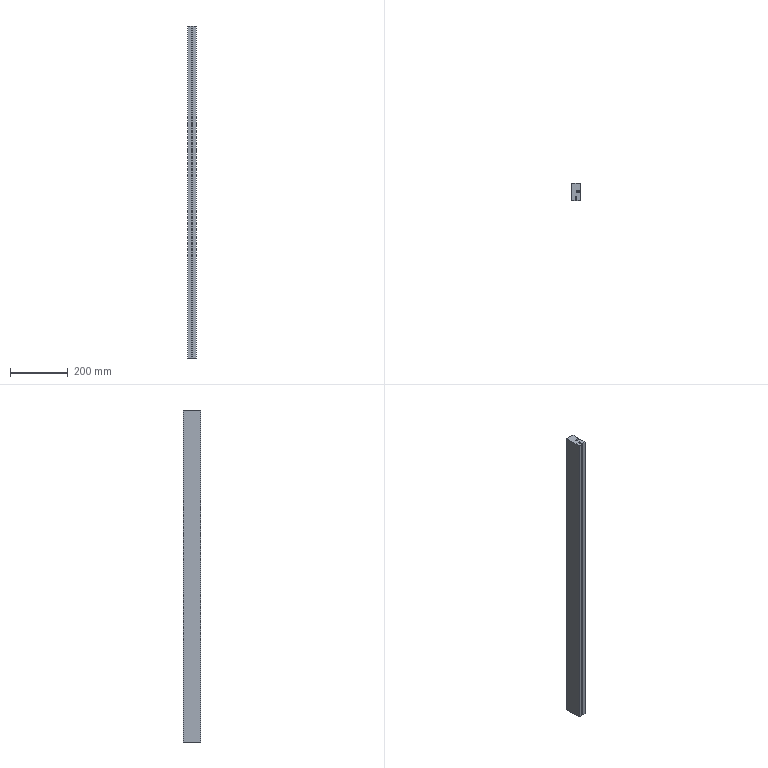Part | STEP file | 750038305 | 1 solid | 14 faces | box 30 x 60 x 1149 mm | volume 1861380 mm3 | plane 14
STEP:
#1=CARTESIAN_POINT('',(0.,0.,1149.));
#2=VERTEX_POINT('',#1);
#3=CARTESIAN_POINT('',(0.,0.,0.));
#4=VERTEX_POINT('',#3);
#5=CARTESIAN_POINT('',(0.,0.,1149.));
#6=DIRECTION('',(0.,0.,-1.));
#7=VECTOR('',#6,1000.);
#8=LINE('',#5,#7);
#9=EDGE_CURVE('',#2,#4,#8,.T.);
#10=ORIENTED_EDGE('',*,*,#9,.F.);
#11=CARTESIAN_POINT('',(0.,60.,1149.));
#12=VERTEX_POINT('',#11);
#13=CARTESIAN_POINT('',(0.,60.,1149.));
#14=DIRECTION('',(0.,-1.,0.));
#15=VECTOR('',#14,1000.);
#16=LINE('',#13,#15);
#17=EDGE_CURVE('',#12,#2,#16,.T.);
#18=ORIENTED_EDGE('',*,*,#17,.F.);
#19=CARTESIAN_POINT('',(0.,60.,0.));
#20=VERTEX_POINT('',#19);
#21=CARTESIAN_POINT('',(0.,60.,1149.));
#22=DIRECTION('',(0.,0.,1.));
#23=VECTOR('',#22,1000.);
#24=LINE('',#21,#23);
#25=EDGE_CURVE('',#20,#12,#24,.T.);
#26=ORIENTED_EDGE('',*,*,#25,.F.);
#27=CARTESIAN_POINT('',(0.,60.,0.));
#28=DIRECTION('',(0.,1.,0.));
#29=VECTOR('',#28,1000.);
#30=LINE('',#27,#29);
#31=EDGE_CURVE('',#4,#20,#30,.T.);
#32=ORIENTED_EDGE('',*,*,#31,.F.);
#33=EDGE_LOOP('',(#10,#18,#26,#32));
#34=FACE_OUTER_BOUND('',#33,.T.);
#35=CARTESIAN_POINT('',(0.,60.,1149.));
#36=DIRECTION('',(1.,0.,0.));
#37=DIRECTION('',(0.,0.,-1.));
#38=AXIS2_PLACEMENT_3D('',#35,#36,#37);
#39=PLANE('',#38);
#40=ADVANCED_FACE('',(#34),#39,.F.);
#41=CARTESIAN_POINT('',(15.,33.,0.));
#42=VERTEX_POINT('',#41);
#43=CARTESIAN_POINT('',(30.,33.,0.));
#44=VERTEX_POINT('',#43);
#45=CARTESIAN_POINT('',(0.,33.,0.));
#46=DIRECTION('',(1.,0.,0.));
#47=VECTOR('',#46,1000.);
#48=LINE('',#45,#47);
#49=EDGE_CURVE('',#42,#44,#48,.T.);
#50=ORIENTED_EDGE('',*,*,#49,.F.);
#51=CARTESIAN_POINT('',(15.,27.,0.));
#52=VERTEX_POINT('',#51);
#53=CARTESIAN_POINT('',(15.,0.,0.));
#54=DIRECTION('',(0.,1.,0.));
#55=VECTOR('',#54,1000.);
#56=LINE('',#53,#55);
#57=EDGE_CURVE('',#52,#42,#56,.T.);
#58=ORIENTED_EDGE('',*,*,#57,.F.);
#59=CARTESIAN_POINT('',(30.,27.,0.));
#60=VERTEX_POINT('',#59);
#61=CARTESIAN_POINT('',(0.,27.,0.));
#62=DIRECTION('',(-1.,0.,0.));
#63=VECTOR('',#62,1000.);
#64=LINE('',#61,#63);
#65=EDGE_CURVE('',#60,#52,#64,.T.);
#66=ORIENTED_EDGE('',*,*,#65,.F.);
#67=CARTESIAN_POINT('',(30.,0.,0.));
#68=VERTEX_POINT('',#67);
#69=CARTESIAN_POINT('',(30.,0.,0.));
#70=DIRECTION('',(0.,1.,0.));
#71=VECTOR('',#70,1000.);
#72=LINE('',#69,#71);
#73=EDGE_CURVE('',#68,#60,#72,.T.);
#74=ORIENTED_EDGE('',*,*,#73,.F.);
#75=CARTESIAN_POINT('',(18.,0.,0.));
#76=VERTEX_POINT('',#75);
#77=CARTESIAN_POINT('',(0.,0.,0.));
#78=DIRECTION('',(1.,0.,0.));
#79=VECTOR('',#78,1000.);
#80=LINE('',#77,#79);
#81=EDGE_CURVE('',#76,#68,#80,.T.);
#82=ORIENTED_EDGE('',*,*,#81,.F.);
#83=CARTESIAN_POINT('',(18.,15.,0.));
#84=VERTEX_POINT('',#83);
#85=CARTESIAN_POINT('',(18.,0.,0.));
#86=DIRECTION('',(0.,-1.,0.));
#87=VECTOR('',#86,1000.);
#88=LINE('',#85,#87);
#89=EDGE_CURVE('',#84,#76,#88,.T.);
#90=ORIENTED_EDGE('',*,*,#89,.F.);
#91=CARTESIAN_POINT('',(12.,15.,0.));
#92=VERTEX_POINT('',#91);
#93=CARTESIAN_POINT('',(0.,15.,0.));
#94=DIRECTION('',(1.,0.,0.));
#95=VECTOR('',#94,1000.);
#96=LINE('',#93,#95);
#97=EDGE_CURVE('',#92,#84,#96,.T.);
#98=ORIENTED_EDGE('',*,*,#97,.F.);
#99=CARTESIAN_POINT('',(12.,0.,0.));
#100=VERTEX_POINT('',#99);
#101=CARTESIAN_POINT('',(12.,0.,0.));
#102=DIRECTION('',(0.,1.,0.));
#103=VECTOR('',#102,1000.);
#104=LINE('',#101,#103);
#105=EDGE_CURVE('',#100,#92,#104,.T.);
#106=ORIENTED_EDGE('',*,*,#105,.F.);
#107=CARTESIAN_POINT('',(0.,0.,0.));
#108=DIRECTION('',(1.,0.,0.));
#109=VECTOR('',#108,1000.);
#110=LINE('',#107,#109);
#111=EDGE_CURVE('',#4,#100,#110,.T.);
#112=ORIENTED_EDGE('',*,*,#111,.F.);
#113=ORIENTED_EDGE('',*,*,#31,.T.);
#114=CARTESIAN_POINT('',(30.,60.,0.));
#115=VERTEX_POINT('',#114);
#116=CARTESIAN_POINT('',(0.,60.,0.));
#117=DIRECTION('',(-1.,0.,0.));
#118=VECTOR('',#117,1000.);
#119=LINE('',#116,#118);
#120=EDGE_CURVE('',#115,#20,#119,.T.);
#121=ORIENTED_EDGE('',*,*,#120,.F.);
#122=CARTESIAN_POINT('',(30.,0.,0.));
#123=DIRECTION('',(0.,1.,0.));
#124=VECTOR('',#123,1000.);
#125=LINE('',#122,#124);
#126=EDGE_CURVE('',#44,#115,#125,.T.);
#127=ORIENTED_EDGE('',*,*,#126,.F.);
#128=EDGE_LOOP('',(#50,#58,#66,#74,#82,#90,#98,#106,#112,#113,#121,#127));
#129=FACE_OUTER_BOUND('',#128,.T.);
#130=CARTESIAN_POINT('',(0.,0.,0.));
#131=DIRECTION('',(0.,0.,1.));
#132=DIRECTION('',(1.,0.,0.));
#133=AXIS2_PLACEMENT_3D('',#130,#131,#132);
#134=PLANE('',#133);
#135=ADVANCED_FACE('',(#129),#134,.F.);
#136=CARTESIAN_POINT('',(12.,0.,1149.));
#137=VERTEX_POINT('',#136);
#138=CARTESIAN_POINT('',(12.,0.,1149.));
#139=DIRECTION('',(0.,0.,-1.));
#140=VECTOR('',#139,1000.);
#141=LINE('',#138,#140);
#142=EDGE_CURVE('',#137,#100,#141,.T.);
#143=ORIENTED_EDGE('',*,*,#142,.F.);
#144=CARTESIAN_POINT('',(0.,0.,1149.));
#145=DIRECTION('',(1.,0.,0.));
#146=VECTOR('',#145,1000.);
#147=LINE('',#144,#146);
#148=EDGE_CURVE('',#2,#137,#147,.T.);
#149=ORIENTED_EDGE('',*,*,#148,.F.);
#150=ORIENTED_EDGE('',*,*,#9,.T.);
#151=ORIENTED_EDGE('',*,*,#111,.T.);
#152=EDGE_LOOP('',(#143,#149,#150,#151));
#153=FACE_OUTER_BOUND('',#152,.T.);
#154=CARTESIAN_POINT('',(0.,0.,1149.));
#155=DIRECTION('',(0.,1.,0.));
#156=DIRECTION('',(0.,0.,1.));
#157=AXIS2_PLACEMENT_3D('',#154,#155,#156);
#158=PLANE('',#157);
#159=ADVANCED_FACE('',(#153),#158,.F.);
#160=CARTESIAN_POINT('',(15.,27.,1149.));
#161=VERTEX_POINT('',#160);
#162=CARTESIAN_POINT('',(15.,33.,1149.));
#163=VERTEX_POINT('',#162);
#164=CARTESIAN_POINT('',(15.,0.,1149.));
#165=DIRECTION('',(0.,1.,0.));
#166=VECTOR('',#165,1000.);
#167=LINE('',#164,#166);
#168=EDGE_CURVE('',#161,#163,#167,.T.);
#169=ORIENTED_EDGE('',*,*,#168,.T.);
#170=CARTESIAN_POINT('',(30.,33.,1149.));
#171=VERTEX_POINT('',#170);
#172=CARTESIAN_POINT('',(0.,33.,1149.));
#173=DIRECTION('',(1.,0.,0.));
#174=VECTOR('',#173,1000.);
#175=LINE('',#172,#174);
#176=EDGE_CURVE('',#163,#171,#175,.T.);
#177=ORIENTED_EDGE('',*,*,#176,.T.);
#178=CARTESIAN_POINT('',(30.,60.,1149.));
#179=VERTEX_POINT('',#178);
#180=CARTESIAN_POINT('',(30.,0.,1149.));
#181=DIRECTION('',(0.,1.,0.));
#182=VECTOR('',#181,1000.);
#183=LINE('',#180,#182);
#184=EDGE_CURVE('',#171,#179,#183,.T.);
#185=ORIENTED_EDGE('',*,*,#184,.T.);
#186=CARTESIAN_POINT('',(0.,60.,1149.));
#187=DIRECTION('',(-1.,0.,0.));
#188=VECTOR('',#187,1000.);
#189=LINE('',#186,#188);
#190=EDGE_CURVE('',#179,#12,#189,.T.);
#191=ORIENTED_EDGE('',*,*,#190,.T.);
#192=ORIENTED_EDGE('',*,*,#17,.T.);
#193=ORIENTED_EDGE('',*,*,#148,.T.);
#194=CARTESIAN_POINT('',(12.,15.,1149.));
#195=VERTEX_POINT('',#194);
#196=CARTESIAN_POINT('',(12.,0.,1149.));
#197=DIRECTION('',(0.,1.,0.));
#198=VECTOR('',#197,1000.);
#199=LINE('',#196,#198);
#200=EDGE_CURVE('',#137,#195,#199,.T.);
#201=ORIENTED_EDGE('',*,*,#200,.T.);
#202=CARTESIAN_POINT('',(18.,15.,1149.));
#203=VERTEX_POINT('',#202);
#204=CARTESIAN_POINT('',(0.,15.,1149.));
#205=DIRECTION('',(1.,0.,0.));
#206=VECTOR('',#205,1000.);
#207=LINE('',#204,#206);
#208=EDGE_CURVE('',#195,#203,#207,.T.);
#209=ORIENTED_EDGE('',*,*,#208,.T.);
#210=CARTESIAN_POINT('',(18.,0.,1149.));
#211=VERTEX_POINT('',#210);
#212=CARTESIAN_POINT('',(18.,0.,1149.));
#213=DIRECTION('',(0.,-1.,0.));
#214=VECTOR('',#213,1000.);
#215=LINE('',#212,#214);
#216=EDGE_CURVE('',#203,#211,#215,.T.);
#217=ORIENTED_EDGE('',*,*,#216,.T.);
#218=CARTESIAN_POINT('',(30.,0.,1149.));
#219=VERTEX_POINT('',#218);
#220=CARTESIAN_POINT('',(0.,0.,1149.));
#221=DIRECTION('',(1.,0.,0.));
#222=VECTOR('',#221,1000.);
#223=LINE('',#220,#222);
#224=EDGE_CURVE('',#211,#219,#223,.T.);
#225=ORIENTED_EDGE('',*,*,#224,.T.);
#226=CARTESIAN_POINT('',(30.,27.,1149.));
#227=VERTEX_POINT('',#226);
#228=CARTESIAN_POINT('',(30.,0.,1149.));
#229=DIRECTION('',(0.,1.,0.));
#230=VECTOR('',#229,1000.);
#231=LINE('',#228,#230);
#232=EDGE_CURVE('',#219,#227,#231,.T.);
#233=ORIENTED_EDGE('',*,*,#232,.T.);
#234=CARTESIAN_POINT('',(0.,27.,1149.));
#235=DIRECTION('',(-1.,0.,0.));
#236=VECTOR('',#235,1000.);
#237=LINE('',#234,#236);
#238=EDGE_CURVE('',#227,#161,#237,.T.);
#239=ORIENTED_EDGE('',*,*,#238,.T.);
#240=EDGE_LOOP('',(#169,#177,#185,#191,#192,#193,#201,#209,#217,#225,#233,#239));
#241=FACE_OUTER_BOUND('',#240,.T.);
#242=CARTESIAN_POINT('',(0.,0.,1149.));
#243=DIRECTION('',(0.,0.,1.));
#244=DIRECTION('',(1.,0.,0.));
#245=AXIS2_PLACEMENT_3D('',#242,#243,#244);
#246=PLANE('',#245);
#247=ADVANCED_FACE('',(#241),#246,.T.);
#248=ORIENTED_EDGE('',*,*,#25,.T.);
#249=ORIENTED_EDGE('',*,*,#190,.F.);
#250=CARTESIAN_POINT('',(30.,60.,1149.));
#251=DIRECTION('',(0.,0.,1.));
#252=VECTOR('',#251,1000.);
#253=LINE('',#250,#252);
#254=EDGE_CURVE('',#115,#179,#253,.T.);
#255=ORIENTED_EDGE('',*,*,#254,.F.);
#256=ORIENTED_EDGE('',*,*,#120,.T.);
#257=EDGE_LOOP('',(#248,#249,#255,#256));
#258=FACE_OUTER_BOUND('',#257,.T.);
#259=CARTESIAN_POINT('',(30.,60.,1149.));
#260=DIRECTION('',(0.,-1.,0.));
#261=DIRECTION('',(0.,0.,-1.));
#262=AXIS2_PLACEMENT_3D('',#259,#260,#261);
#263=PLANE('',#262);
#264=ADVANCED_FACE('',(#258),#263,.F.);
#265=ORIENTED_EDGE('',*,*,#254,.T.);
#266=ORIENTED_EDGE('',*,*,#184,.F.);
#267=CARTESIAN_POINT('',(30.,33.,1149.));
#268=DIRECTION('',(0.,0.,1.));
#269=VECTOR('',#268,1000.);
#270=LINE('',#267,#269);
#271=EDGE_CURVE('',#44,#171,#270,.T.);
#272=ORIENTED_EDGE('',*,*,#271,.F.);
#273=ORIENTED_EDGE('',*,*,#126,.T.);
#274=EDGE_LOOP('',(#265,#266,#272,#273));
#275=FACE_OUTER_BOUND('',#274,.T.);
#276=CARTESIAN_POINT('',(30.,33.,1149.));
#277=DIRECTION('',(-1.,0.,0.));
#278=DIRECTION('',(0.,0.,1.));
#279=AXIS2_PLACEMENT_3D('',#276,#277,#278);
#280=PLANE('',#279);
#281=ADVANCED_FACE('',(#275),#280,.F.);
#282=ORIENTED_EDGE('',*,*,#271,.T.);
#283=ORIENTED_EDGE('',*,*,#176,.F.);
#284=CARTESIAN_POINT('',(15.,33.,1149.));
#285=DIRECTION('',(0.,0.,1.));
#286=VECTOR('',#285,1000.);
#287=LINE('',#284,#286);
#288=EDGE_CURVE('',#42,#163,#287,.T.);
#289=ORIENTED_EDGE('',*,*,#288,.F.);
#290=ORIENTED_EDGE('',*,*,#49,.T.);
#291=EDGE_LOOP('',(#282,#283,#289,#290));
#292=FACE_OUTER_BOUND('',#291,.T.);
#293=CARTESIAN_POINT('',(15.,33.,1149.));
#294=DIRECTION('',(0.,1.,0.));
#295=DIRECTION('',(0.,0.,1.));
#296=AXIS2_PLACEMENT_3D('',#293,#294,#295);
#297=PLANE('',#296);
#298=ADVANCED_FACE('',(#292),#297,.F.);
#299=ORIENTED_EDGE('',*,*,#288,.T.);
#300=ORIENTED_EDGE('',*,*,#168,.F.);
#301=CARTESIAN_POINT('',(15.,27.,1149.));
#302=DIRECTION('',(0.,0.,1.));
#303=VECTOR('',#302,1000.);
#304=LINE('',#301,#303);
#305=EDGE_CURVE('',#52,#161,#304,.T.);
#306=ORIENTED_EDGE('',*,*,#305,.F.);
#307=ORIENTED_EDGE('',*,*,#57,.T.);
#308=EDGE_LOOP('',(#299,#300,#306,#307));
#309=FACE_OUTER_BOUND('',#308,.T.);
#310=CARTESIAN_POINT('',(15.,27.,1149.));
#311=DIRECTION('',(-1.,0.,0.));
#312=DIRECTION('',(0.,0.,1.));
#313=AXIS2_PLACEMENT_3D('',#310,#311,#312);
#314=PLANE('',#313);
#315=ADVANCED_FACE('',(#309),#314,.F.);
#316=ORIENTED_EDGE('',*,*,#305,.T.);
#317=ORIENTED_EDGE('',*,*,#238,.F.);
#318=CARTESIAN_POINT('',(30.,27.,1149.));
#319=DIRECTION('',(0.,0.,1.));
#320=VECTOR('',#319,1000.);
#321=LINE('',#318,#320);
#322=EDGE_CURVE('',#60,#227,#321,.T.);
#323=ORIENTED_EDGE('',*,*,#322,.F.);
#324=ORIENTED_EDGE('',*,*,#65,.T.);
#325=EDGE_LOOP('',(#316,#317,#323,#324));
#326=FACE_OUTER_BOUND('',#325,.T.);
#327=CARTESIAN_POINT('',(30.,27.,1149.));
#328=DIRECTION('',(0.,-1.,0.));
#329=DIRECTION('',(0.,0.,-1.));
#330=AXIS2_PLACEMENT_3D('',#327,#328,#329);
#331=PLANE('',#330);
#332=ADVANCED_FACE('',(#326),#331,.F.);
#333=ORIENTED_EDGE('',*,*,#322,.T.);
#334=ORIENTED_EDGE('',*,*,#232,.F.);
#335=CARTESIAN_POINT('',(30.,0.,1149.));
#336=DIRECTION('',(0.,0.,1.));
#337=VECTOR('',#336,1000.);
#338=LINE('',#335,#337);
#339=EDGE_CURVE('',#68,#219,#338,.T.);
#340=ORIENTED_EDGE('',*,*,#339,.F.);
#341=ORIENTED_EDGE('',*,*,#73,.T.);
#342=EDGE_LOOP('',(#333,#334,#340,#341));
#343=FACE_OUTER_BOUND('',#342,.T.);
#344=CARTESIAN_POINT('',(30.,0.,1149.));
#345=DIRECTION('',(-1.,0.,0.));
#346=DIRECTION('',(0.,-1.,0.));
#347=AXIS2_PLACEMENT_3D('',#344,#345,#346);
#348=PLANE('',#347);
#349=ADVANCED_FACE('',(#343),#348,.F.);
#350=ORIENTED_EDGE('',*,*,#339,.T.);
#351=ORIENTED_EDGE('',*,*,#224,.F.);
#352=CARTESIAN_POINT('',(18.,0.,1149.));
#353=DIRECTION('',(0.,0.,1.));
#354=VECTOR('',#353,1000.);
#355=LINE('',#352,#354);
#356=EDGE_CURVE('',#76,#211,#355,.T.);
#357=ORIENTED_EDGE('',*,*,#356,.F.);
#358=ORIENTED_EDGE('',*,*,#81,.T.);
#359=EDGE_LOOP('',(#350,#351,#357,#358));
#360=FACE_OUTER_BOUND('',#359,.T.);
#361=CARTESIAN_POINT('',(18.,0.,1149.));
#362=DIRECTION('',(0.,1.,0.));
#363=DIRECTION('',(-1.,0.,0.));
#364=AXIS2_PLACEMENT_3D('',#361,#362,#363);
#365=PLANE('',#364);
#366=ADVANCED_FACE('',(#360),#365,.F.);
#367=ORIENTED_EDGE('',*,*,#356,.T.);
#368=ORIENTED_EDGE('',*,*,#216,.F.);
#369=CARTESIAN_POINT('',(18.,15.,1149.));
#370=DIRECTION('',(0.,0.,1.));
#371=VECTOR('',#370,1000.);
#372=LINE('',#369,#371);
#373=EDGE_CURVE('',#84,#203,#372,.T.);
#374=ORIENTED_EDGE('',*,*,#373,.F.);
#375=ORIENTED_EDGE('',*,*,#89,.T.);
#376=EDGE_LOOP('',(#367,#368,#374,#375));
#377=FACE_OUTER_BOUND('',#376,.T.);
#378=CARTESIAN_POINT('',(18.,15.,1149.));
#379=DIRECTION('',(1.,0.,0.));
#380=DIRECTION('',(0.,1.,0.));
#381=AXIS2_PLACEMENT_3D('',#378,#379,#380);
#382=PLANE('',#381);
#383=ADVANCED_FACE('',(#377),#382,.F.);
#384=ORIENTED_EDGE('',*,*,#373,.T.);
#385=ORIENTED_EDGE('',*,*,#208,.F.);
#386=CARTESIAN_POINT('',(12.,15.,1149.));
#387=DIRECTION('',(0.,0.,1.));
#388=VECTOR('',#387,1000.);
#389=LINE('',#386,#388);
#390=EDGE_CURVE('',#92,#195,#389,.T.);
#391=ORIENTED_EDGE('',*,*,#390,.F.);
#392=ORIENTED_EDGE('',*,*,#97,.T.);
#393=EDGE_LOOP('',(#384,#385,#391,#392));
#394=FACE_OUTER_BOUND('',#393,.T.);
#395=CARTESIAN_POINT('',(12.,15.,1149.));
#396=DIRECTION('',(0.,1.,0.));
#397=DIRECTION('',(-1.,0.,0.));
#398=AXIS2_PLACEMENT_3D('',#395,#396,#397);
#399=PLANE('',#398);
#400=ADVANCED_FACE('',(#394),#399,.F.);
#401=ORIENTED_EDGE('',*,*,#390,.T.);
#402=ORIENTED_EDGE('',*,*,#200,.F.);
#403=ORIENTED_EDGE('',*,*,#142,.T.);
#404=ORIENTED_EDGE('',*,*,#105,.T.);
#405=EDGE_LOOP('',(#401,#402,#403,#404));
#406=FACE_OUTER_BOUND('',#405,.T.);
#407=CARTESIAN_POINT('',(12.,0.,1149.));
#408=DIRECTION('',(-1.,0.,0.));
#409=DIRECTION('',(0.,0.,1.));
#410=AXIS2_PLACEMENT_3D('',#407,#408,#409);
#411=PLANE('',#410);
#412=ADVANCED_FACE('',(#406),#411,.F.);
#413=CLOSED_SHELL('',(#40,#135,#159,#247,#264,#281,#298,#315,#332,#349,#366,#383,#400,#412));
#414=MANIFOLD_SOLID_BREP('',#413);
#415=CARTESIAN_POINT('',(0.,0.,0.));
#416=DIRECTION('',(0.,0.,1.));
#417=DIRECTION('',(1.,0.,0.));
#418=AXIS2_PLACEMENT_3D('',#415,#416,#417);
#419=(LENGTH_UNIT()NAMED_UNIT(*)SI_UNIT(.MILLI.,.METRE.));
#420=UNCERTAINTY_MEASURE_WITH_UNIT(LENGTH_MEASURE(0.00001),#419,'','');
#421=(NAMED_UNIT(*)PLANE_ANGLE_UNIT()SI_UNIT($,.RADIAN.));
#422=(NAMED_UNIT(*)SI_UNIT($,.STERADIAN.)SOLID_ANGLE_UNIT());
#423=(GEOMETRIC_REPRESENTATION_CONTEXT(3)GLOBAL_UNCERTAINTY_ASSIGNED_CONTEXT((#420))GLOBAL_UNIT_ASSIGNED_CONTEXT((#419,#421,#422))REPRESENTATION_CONTEXT('',''));
#424=ADVANCED_BREP_SHAPE_REPRESENTATION('',(#414,#418),#423);